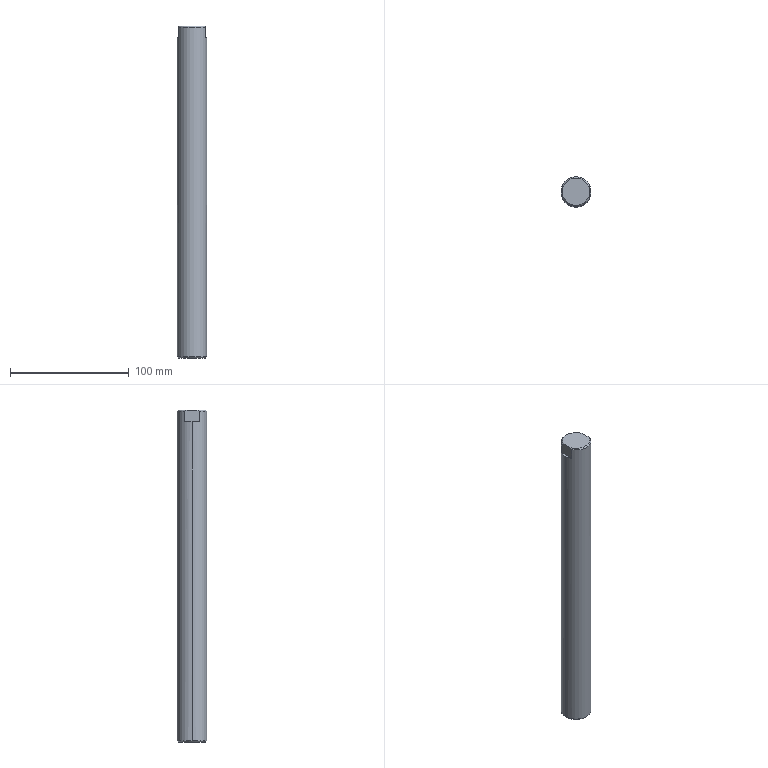Part | SolidWorks | features BaseBody 1 | 1 solid | 16 faces | box 25 x 25 x 280 mm | volume 136306 mm3 | cone 6 | plane 6 | cylinder 4 | commonest cylinder face diameters 6.8 x2 25 x2
STEP:
#1=CARTESIAN_POINT('',(3.4,0.,22.25));
#2=VERTEX_POINT('',#1);
#3=CARTESIAN_POINT('',(-3.4,0.,22.25));
#4=VERTEX_POINT('',#3);
#5=CARTESIAN_POINT('',(0.,0.,22.25));
#6=DIRECTION('',(0.,0.,-1.));
#7=DIRECTION('',(-1.,0.,0.));
#8=AXIS2_PLACEMENT_3D('',#5,#6,#7);
#9=CIRCLE('',#8,3.4);
#10=EDGE_CURVE('',#2,#4,#9,.T.);
#11=ORIENTED_EDGE('',*,*,#10,.F.);
#12=CARTESIAN_POINT('',(3.4,0.,0.));
#13=VERTEX_POINT('',#12);
#14=CARTESIAN_POINT('',(3.4,0.,0.));
#15=DIRECTION('',(0.,0.,-1.));
#16=VECTOR('',#15,1000.);
#17=LINE('',#14,#16);
#18=EDGE_CURVE('',#2,#13,#17,.T.);
#19=ORIENTED_EDGE('',*,*,#18,.T.);
#20=CARTESIAN_POINT('',(-3.4,0.,0.));
#21=VERTEX_POINT('',#20);
#22=CARTESIAN_POINT('',(0.,0.,0.));
#23=DIRECTION('',(0.,0.,-1.));
#24=DIRECTION('',(-1.,0.,0.));
#25=AXIS2_PLACEMENT_3D('',#22,#23,#24);
#26=CIRCLE('',#25,3.4);
#27=EDGE_CURVE('',#13,#21,#26,.T.);
#28=ORIENTED_EDGE('',*,*,#27,.T.);
#29=CARTESIAN_POINT('',(-3.4,0.,0.));
#30=DIRECTION('',(0.,0.,-1.));
#31=VECTOR('',#30,1000.);
#32=LINE('',#29,#31);
#33=EDGE_CURVE('',#4,#21,#32,.T.);
#34=ORIENTED_EDGE('',*,*,#33,.F.);
#35=EDGE_LOOP('',(#11,#19,#28,#34));
#36=FACE_OUTER_BOUND('',#35,.T.);
#37=CARTESIAN_POINT('',(0.,0.,0.));
#38=DIRECTION('',(0.,0.,-1.));
#39=DIRECTION('',(-1.,0.,0.));
#40=AXIS2_PLACEMENT_3D('',#37,#38,#39);
#41=CYLINDRICAL_SURFACE('',#40,3.4);
#42=ADVANCED_FACE('',(#36),#41,.F.);
#43=CARTESIAN_POINT('',(0.,0.,24.293));
#44=VERTEX_POINT('',#43);
#45=CARTESIAN_POINT('',(-3.4,0.,22.25));
#46=DIRECTION('',(-0.8572,0.,-0.515));
#47=VECTOR('',#46,1000.);
#48=LINE('',#45,#47);
#49=EDGE_CURVE('',#44,#4,#48,.T.);
#50=ORIENTED_EDGE('',*,*,#49,.F.);
#51=CARTESIAN_POINT('',(3.4,0.,22.25));
#52=DIRECTION('',(0.8572,0.,-0.515));
#53=VECTOR('',#52,1000.);
#54=LINE('',#51,#53);
#55=EDGE_CURVE('',#44,#2,#54,.T.);
#56=ORIENTED_EDGE('',*,*,#55,.T.);
#57=ORIENTED_EDGE('',*,*,#10,.T.);
#58=EDGE_LOOP('',(#50,#56,#57));
#59=FACE_OUTER_BOUND('',#58,.T.);
#60=CARTESIAN_POINT('',(0.,0.,22.25));
#61=DIRECTION('',(0.,0.,-1.));
#62=DIRECTION('',(-1.,0.,0.));
#63=AXIS2_PLACEMENT_3D('',#60,#61,#62);
#64=CONICAL_SURFACE('',#63,3.4,1.03);
#65=ADVANCED_FACE('',(#59),#64,.F.);
#66=CARTESIAN_POINT('',(-11.5,0.,0.));
#67=VERTEX_POINT('',#66);
#68=CARTESIAN_POINT('',(11.5,0.,0.));
#69=VERTEX_POINT('',#68);
#70=CARTESIAN_POINT('',(0.,0.,0.));
#71=DIRECTION('',(0.,0.,-1.));
#72=DIRECTION('',(1.,0.,0.));
#73=AXIS2_PLACEMENT_3D('',#70,#71,#72);
#74=CIRCLE('',#73,11.5);
#75=EDGE_CURVE('',#67,#69,#74,.T.);
#76=ORIENTED_EDGE('',*,*,#75,.F.);
#77=CARTESIAN_POINT('',(-12.5,0.,1.));
#78=VERTEX_POINT('',#77);
#79=CARTESIAN_POINT('',(-12.5,0.,1.));
#80=DIRECTION('',(-0.7071,0.,0.7071));
#81=VECTOR('',#80,1000.);
#82=LINE('',#79,#81);
#83=EDGE_CURVE('',#67,#78,#82,.T.);
#84=ORIENTED_EDGE('',*,*,#83,.T.);
#85=CARTESIAN_POINT('',(12.5,0.,1.));
#86=VERTEX_POINT('',#85);
#87=CARTESIAN_POINT('',(0.,0.,1.));
#88=DIRECTION('',(0.,0.,1.));
#89=DIRECTION('',(1.,0.,0.));
#90=AXIS2_PLACEMENT_3D('',#87,#88,#89);
#91=CIRCLE('',#90,12.5);
#92=EDGE_CURVE('',#86,#78,#91,.T.);
#93=ORIENTED_EDGE('',*,*,#92,.F.);
#94=CARTESIAN_POINT('',(12.5,0.,1.));
#95=DIRECTION('',(0.7071,0.,0.7071));
#96=VECTOR('',#95,1000.);
#97=LINE('',#94,#96);
#98=EDGE_CURVE('',#69,#86,#97,.T.);
#99=ORIENTED_EDGE('',*,*,#98,.F.);
#100=EDGE_LOOP('',(#76,#84,#93,#99));
#101=FACE_OUTER_BOUND('',#100,.T.);
#102=CARTESIAN_POINT('',(0.,0.,1.));
#103=DIRECTION('',(0.,0.,1.));
#104=DIRECTION('',(1.,0.,0.));
#105=AXIS2_PLACEMENT_3D('',#102,#103,#104);
#106=CONICAL_SURFACE('',#105,12.5,0.7854);
#107=ADVANCED_FACE('',(#101),#106,.T.);
#108=CARTESIAN_POINT('',(12.5,0.,270.));
#109=VERTEX_POINT('',#108);
#110=CARTESIAN_POINT('',(11.,5.937,270.));
#111=VERTEX_POINT('',#110);
#112=CARTESIAN_POINT('',(0.,0.,270.));
#113=DIRECTION('',(0.,0.,1.));
#114=DIRECTION('',(1.,0.,0.));
#115=AXIS2_PLACEMENT_3D('',#112,#113,#114);
#116=CIRCLE('',#115,12.5);
#117=EDGE_CURVE('',#109,#111,#116,.T.);
#118=ORIENTED_EDGE('',*,*,#117,.F.);
#119=CARTESIAN_POINT('',(12.5,0.,280.));
#120=DIRECTION('',(0.,0.,-1.));
#121=VECTOR('',#120,1000.);
#122=LINE('',#119,#121);
#123=EDGE_CURVE('',#109,#86,#122,.T.);
#124=ORIENTED_EDGE('',*,*,#123,.T.);
#125=ORIENTED_EDGE('',*,*,#92,.T.);
#126=CARTESIAN_POINT('',(-12.5,0.,270.));
#127=VERTEX_POINT('',#126);
#128=CARTESIAN_POINT('',(-12.5,0.,280.));
#129=DIRECTION('',(0.,0.,-1.));
#130=VECTOR('',#129,1000.);
#131=LINE('',#128,#130);
#132=EDGE_CURVE('',#127,#78,#131,.T.);
#133=ORIENTED_EDGE('',*,*,#132,.F.);
#134=CARTESIAN_POINT('',(-11.,5.937,270.));
#135=VERTEX_POINT('',#134);
#136=CARTESIAN_POINT('',(0.,0.,270.));
#137=DIRECTION('',(0.,0.,1.));
#138=DIRECTION('',(1.,0.,0.));
#139=AXIS2_PLACEMENT_3D('',#136,#137,#138);
#140=CIRCLE('',#139,12.5);
#141=EDGE_CURVE('',#135,#127,#140,.T.);
#142=ORIENTED_EDGE('',*,*,#141,.F.);
#143=CARTESIAN_POINT('',(-11.,5.937,279.));
#144=VERTEX_POINT('',#143);
#145=CARTESIAN_POINT('',(-11.,5.937,280.));
#146=DIRECTION('',(0.,0.,1.));
#147=VECTOR('',#146,1000.);
#148=LINE('',#145,#147);
#149=EDGE_CURVE('',#135,#144,#148,.T.);
#150=ORIENTED_EDGE('',*,*,#149,.T.);
#151=CARTESIAN_POINT('',(11.,5.937,279.));
#152=VERTEX_POINT('',#151);
#153=CARTESIAN_POINT('',(0.,0.,279.));
#154=DIRECTION('',(0.,0.,-1.));
#155=DIRECTION('',(1.,0.,0.));
#156=AXIS2_PLACEMENT_3D('',#153,#154,#155);
#157=CIRCLE('',#156,12.5);
#158=EDGE_CURVE('',#144,#152,#157,.T.);
#159=ORIENTED_EDGE('',*,*,#158,.T.);
#160=CARTESIAN_POINT('',(11.,5.937,280.));
#161=DIRECTION('',(0.,0.,-1.));
#162=VECTOR('',#161,1000.);
#163=LINE('',#160,#162);
#164=EDGE_CURVE('',#152,#111,#163,.T.);
#165=ORIENTED_EDGE('',*,*,#164,.T.);
#166=EDGE_LOOP('',(#118,#124,#125,#133,#142,#150,#159,#165));
#167=FACE_OUTER_BOUND('',#166,.T.);
#168=CARTESIAN_POINT('',(0.,0.,280.));
#169=DIRECTION('',(0.,0.,-1.));
#170=DIRECTION('',(-1.,0.,0.));
#171=AXIS2_PLACEMENT_3D('',#168,#169,#170);
#172=CYLINDRICAL_SURFACE('',#171,12.5);
#173=ADVANCED_FACE('',(#167),#172,.T.);
#174=CARTESIAN_POINT('',(11.,3.354,280.));
#175=VERTEX_POINT('',#174);
#176=CARTESIAN_POINT('',(11.,5.937,279.));
#177=CARTESIAN_POINT('',(11.,5.097,279.399));
#178=CARTESIAN_POINT('',(11.,4.239,279.742));
#179=CARTESIAN_POINT('',(11.,3.354,280.));
#180=B_SPLINE_CURVE_WITH_KNOTS('',3,(#176,#177,#178,#179),.UNSPECIFIED.,.F.,.F.,(4,4),(0.02005,0.02282),.UNSPECIFIED.);
#181=EDGE_CURVE('',#152,#175,#180,.T.);
#182=ORIENTED_EDGE('',*,*,#181,.F.);
#183=ORIENTED_EDGE('',*,*,#158,.F.);
#184=CARTESIAN_POINT('',(-11.,3.354,280.));
#185=VERTEX_POINT('',#184);
#186=CARTESIAN_POINT('',(-11.,3.354,280.));
#187=CARTESIAN_POINT('',(-11.,4.247,279.739));
#188=CARTESIAN_POINT('',(-11.,5.104,279.396));
#189=CARTESIAN_POINT('',(-11.,5.937,279.));
#190=B_SPLINE_CURVE_WITH_KNOTS('',3,(#186,#187,#188,#189),.UNSPECIFIED.,.F.,.F.,(4,4),(0.02963,0.03241),.UNSPECIFIED.);
#191=EDGE_CURVE('',#185,#144,#190,.T.);
#192=ORIENTED_EDGE('',*,*,#191,.F.);
#193=CARTESIAN_POINT('',(0.,0.,280.));
#194=DIRECTION('',(0.,0.,1.));
#195=DIRECTION('',(1.,0.,0.));
#196=AXIS2_PLACEMENT_3D('',#193,#194,#195);
#197=CIRCLE('',#196,11.5);
#198=EDGE_CURVE('',#175,#185,#197,.T.);
#199=ORIENTED_EDGE('',*,*,#198,.F.);
#200=EDGE_LOOP('',(#182,#183,#192,#199));
#201=FACE_OUTER_BOUND('',#200,.T.);
#202=CARTESIAN_POINT('',(0.,0.,280.));
#203=DIRECTION('',(0.,0.,-1.));
#204=DIRECTION('',(-1.,0.,0.));
#205=AXIS2_PLACEMENT_3D('',#202,#203,#204);
#206=CONICAL_SURFACE('',#205,11.5,0.7854);
#207=ADVANCED_FACE('',(#201),#206,.T.);
#208=ORIENTED_EDGE('',*,*,#123,.F.);
#209=CARTESIAN_POINT('',(11.,-5.937,270.));
#210=VERTEX_POINT('',#209);
#211=CARTESIAN_POINT('',(0.,0.,270.));
#212=DIRECTION('',(0.,0.,1.));
#213=DIRECTION('',(1.,0.,0.));
#214=AXIS2_PLACEMENT_3D('',#211,#212,#213);
#215=CIRCLE('',#214,12.5);
#216=EDGE_CURVE('',#210,#109,#215,.T.);
#217=ORIENTED_EDGE('',*,*,#216,.F.);
#218=CARTESIAN_POINT('',(11.,-5.937,279.));
#219=VERTEX_POINT('',#218);
#220=CARTESIAN_POINT('',(11.,-5.937,280.));
#221=DIRECTION('',(0.,0.,1.));
#222=VECTOR('',#221,1000.);
#223=LINE('',#220,#222);
#224=EDGE_CURVE('',#210,#219,#223,.T.);
#225=ORIENTED_EDGE('',*,*,#224,.T.);
#226=CARTESIAN_POINT('',(-11.,-5.937,279.));
#227=VERTEX_POINT('',#226);
#228=CARTESIAN_POINT('',(0.,0.,279.));
#229=DIRECTION('',(0.,0.,-1.));
#230=DIRECTION('',(1.,0.,0.));
#231=AXIS2_PLACEMENT_3D('',#228,#229,#230);
#232=CIRCLE('',#231,12.5);
#233=EDGE_CURVE('',#219,#227,#232,.T.);
#234=ORIENTED_EDGE('',*,*,#233,.T.);
#235=CARTESIAN_POINT('',(-11.,-5.937,270.));
#236=VERTEX_POINT('',#235);
#237=CARTESIAN_POINT('',(-11.,-5.937,280.));
#238=DIRECTION('',(0.,0.,-1.));
#239=VECTOR('',#238,1000.);
#240=LINE('',#237,#239);
#241=EDGE_CURVE('',#227,#236,#240,.T.);
#242=ORIENTED_EDGE('',*,*,#241,.T.);
#243=CARTESIAN_POINT('',(0.,0.,270.));
#244=DIRECTION('',(0.,0.,1.));
#245=DIRECTION('',(1.,0.,0.));
#246=AXIS2_PLACEMENT_3D('',#243,#244,#245);
#247=CIRCLE('',#246,12.5);
#248=EDGE_CURVE('',#127,#236,#247,.T.);
#249=ORIENTED_EDGE('',*,*,#248,.F.);
#250=ORIENTED_EDGE('',*,*,#132,.T.);
#251=CARTESIAN_POINT('',(0.,0.,1.));
#252=DIRECTION('',(0.,0.,1.));
#253=DIRECTION('',(1.,0.,0.));
#254=AXIS2_PLACEMENT_3D('',#251,#252,#253);
#255=CIRCLE('',#254,12.5);
#256=EDGE_CURVE('',#78,#86,#255,.T.);
#257=ORIENTED_EDGE('',*,*,#256,.T.);
#258=EDGE_LOOP('',(#208,#217,#225,#234,#242,#249,#250,#257));
#259=FACE_OUTER_BOUND('',#258,.T.);
#260=CARTESIAN_POINT('',(0.,0.,280.));
#261=DIRECTION('',(0.,0.,-1.));
#262=DIRECTION('',(-1.,0.,0.));
#263=AXIS2_PLACEMENT_3D('',#260,#261,#262);
#264=CYLINDRICAL_SURFACE('',#263,12.5);
#265=ADVANCED_FACE('',(#259),#264,.T.);
#266=CARTESIAN_POINT('',(11.,-3.354,280.));
#267=VERTEX_POINT('',#266);
#268=CARTESIAN_POINT('',(11.,10.,280.));
#269=DIRECTION('',(0.,-1.,0.));
#270=VECTOR('',#269,1000.);
#271=LINE('',#268,#270);
#272=EDGE_CURVE('',#175,#267,#271,.T.);
#273=ORIENTED_EDGE('',*,*,#272,.F.);
#274=ORIENTED_EDGE('',*,*,#198,.T.);
#275=CARTESIAN_POINT('',(-11.,-3.354,280.));
#276=VERTEX_POINT('',#275);
#277=CARTESIAN_POINT('',(-11.,10.,280.));
#278=DIRECTION('',(0.,1.,0.));
#279=VECTOR('',#278,1000.);
#280=LINE('',#277,#279);
#281=EDGE_CURVE('',#276,#185,#280,.T.);
#282=ORIENTED_EDGE('',*,*,#281,.F.);
#283=CARTESIAN_POINT('',(0.,0.,280.));
#284=DIRECTION('',(0.,0.,1.));
#285=DIRECTION('',(1.,0.,0.));
#286=AXIS2_PLACEMENT_3D('',#283,#284,#285);
#287=CIRCLE('',#286,11.5);
#288=EDGE_CURVE('',#276,#267,#287,.T.);
#289=ORIENTED_EDGE('',*,*,#288,.T.);
#290=EDGE_LOOP('',(#273,#274,#282,#289));
#291=FACE_OUTER_BOUND('',#290,.T.);
#292=CARTESIAN_POINT('',(0.,0.,280.));
#293=DIRECTION('',(0.,0.,1.));
#294=DIRECTION('',(1.,0.,0.));
#295=AXIS2_PLACEMENT_3D('',#292,#293,#294);
#296=PLANE('',#295);
#297=ADVANCED_FACE('',(#291),#296,.T.);
#298=CARTESIAN_POINT('',(0.,0.,0.));
#299=DIRECTION('',(0.,0.,-1.));
#300=DIRECTION('',(-1.,0.,0.));
#301=AXIS2_PLACEMENT_3D('',#298,#299,#300);
#302=CIRCLE('',#301,3.4);
#303=EDGE_CURVE('',#21,#13,#302,.T.);
#304=ORIENTED_EDGE('',*,*,#303,.F.);
#305=ORIENTED_EDGE('',*,*,#27,.F.);
#306=EDGE_LOOP('',(#304,#305));
#307=FACE_BOUND('',#306,.T.);
#308=CARTESIAN_POINT('',(0.,0.,0.));
#309=DIRECTION('',(0.,0.,-1.));
#310=DIRECTION('',(1.,0.,0.));
#311=AXIS2_PLACEMENT_3D('',#308,#309,#310);
#312=CIRCLE('',#311,11.5);
#313=EDGE_CURVE('',#69,#67,#312,.T.);
#314=ORIENTED_EDGE('',*,*,#313,.T.);
#315=ORIENTED_EDGE('',*,*,#75,.T.);
#316=EDGE_LOOP('',(#314,#315));
#317=FACE_OUTER_BOUND('',#316,.T.);
#318=CARTESIAN_POINT('',(0.,0.,0.));
#319=DIRECTION('',(0.,0.,1.));
#320=DIRECTION('',(1.,0.,0.));
#321=AXIS2_PLACEMENT_3D('',#318,#319,#320);
#322=PLANE('',#321);
#323=ADVANCED_FACE('',(#307,#317),#322,.F.);
#324=ORIENTED_EDGE('',*,*,#83,.F.);
#325=ORIENTED_EDGE('',*,*,#313,.F.);
#326=ORIENTED_EDGE('',*,*,#98,.T.);
#327=ORIENTED_EDGE('',*,*,#256,.F.);
#328=EDGE_LOOP('',(#324,#325,#326,#327));
#329=FACE_OUTER_BOUND('',#328,.T.);
#330=CARTESIAN_POINT('',(0.,0.,1.));
#331=DIRECTION('',(0.,0.,1.));
#332=DIRECTION('',(1.,0.,0.));
#333=AXIS2_PLACEMENT_3D('',#330,#331,#332);
#334=CONICAL_SURFACE('',#333,12.5,0.7854);
#335=ADVANCED_FACE('',(#329),#334,.T.);
#336=CARTESIAN_POINT('',(11.,-3.354,280.));
#337=CARTESIAN_POINT('',(11.,-4.247,279.739));
#338=CARTESIAN_POINT('',(11.,-5.104,279.396));
#339=CARTESIAN_POINT('',(11.,-5.937,279.));
#340=B_SPLINE_CURVE_WITH_KNOTS('',3,(#336,#337,#338,#339),.UNSPECIFIED.,.F.,.F.,(4,4),(0.02963,0.03241),.UNSPECIFIED.);
#341=EDGE_CURVE('',#267,#219,#340,.T.);
#342=ORIENTED_EDGE('',*,*,#341,.F.);
#343=ORIENTED_EDGE('',*,*,#288,.F.);
#344=CARTESIAN_POINT('',(-11.,-5.937,279.));
#345=CARTESIAN_POINT('',(-11.,-5.097,279.399));
#346=CARTESIAN_POINT('',(-11.,-4.239,279.742));
#347=CARTESIAN_POINT('',(-11.,-3.354,280.));
#348=B_SPLINE_CURVE_WITH_KNOTS('',3,(#344,#345,#346,#347),.UNSPECIFIED.,.F.,.F.,(4,4),(0.02005,0.02282),.UNSPECIFIED.);
#349=EDGE_CURVE('',#227,#276,#348,.T.);
#350=ORIENTED_EDGE('',*,*,#349,.F.);
#351=ORIENTED_EDGE('',*,*,#233,.F.);
#352=EDGE_LOOP('',(#342,#343,#350,#351));
#353=FACE_OUTER_BOUND('',#352,.T.);
#354=CARTESIAN_POINT('',(0.,0.,280.));
#355=DIRECTION('',(0.,0.,-1.));
#356=DIRECTION('',(-1.,0.,0.));
#357=AXIS2_PLACEMENT_3D('',#354,#355,#356);
#358=CONICAL_SURFACE('',#357,11.5,0.7854);
#359=ADVANCED_FACE('',(#353),#358,.T.);
#360=ORIENTED_EDGE('',*,*,#55,.F.);
#361=ORIENTED_EDGE('',*,*,#49,.T.);
#362=CARTESIAN_POINT('',(0.,0.,22.25));
#363=DIRECTION('',(0.,0.,-1.));
#364=DIRECTION('',(-1.,0.,0.));
#365=AXIS2_PLACEMENT_3D('',#362,#363,#364);
#366=CIRCLE('',#365,3.4);
#367=EDGE_CURVE('',#4,#2,#366,.T.);
#368=ORIENTED_EDGE('',*,*,#367,.T.);
#369=EDGE_LOOP('',(#360,#361,#368));
#370=FACE_OUTER_BOUND('',#369,.T.);
#371=CARTESIAN_POINT('',(0.,0.,22.25));
#372=DIRECTION('',(0.,0.,-1.));
#373=DIRECTION('',(-1.,0.,0.));
#374=AXIS2_PLACEMENT_3D('',#371,#372,#373);
#375=CONICAL_SURFACE('',#374,3.4,1.03);
#376=ADVANCED_FACE('',(#370),#375,.F.);
#377=ORIENTED_EDGE('',*,*,#18,.F.);
#378=ORIENTED_EDGE('',*,*,#367,.F.);
#379=ORIENTED_EDGE('',*,*,#33,.T.);
#380=ORIENTED_EDGE('',*,*,#303,.T.);
#381=EDGE_LOOP('',(#377,#378,#379,#380));
#382=FACE_OUTER_BOUND('',#381,.T.);
#383=CARTESIAN_POINT('',(0.,0.,0.));
#384=DIRECTION('',(0.,0.,-1.));
#385=DIRECTION('',(-1.,0.,0.));
#386=AXIS2_PLACEMENT_3D('',#383,#384,#385);
#387=CYLINDRICAL_SURFACE('',#386,3.4);
#388=ADVANCED_FACE('',(#382),#387,.F.);
#389=ORIENTED_EDGE('',*,*,#141,.T.);
#390=ORIENTED_EDGE('',*,*,#248,.T.);
#391=CARTESIAN_POINT('',(-11.,10.,270.));
#392=DIRECTION('',(0.,1.,0.));
#393=VECTOR('',#392,1000.);
#394=LINE('',#391,#393);
#395=EDGE_CURVE('',#236,#135,#394,.T.);
#396=ORIENTED_EDGE('',*,*,#395,.T.);
#397=EDGE_LOOP('',(#389,#390,#396));
#398=FACE_OUTER_BOUND('',#397,.T.);
#399=CARTESIAN_POINT('',(0.,0.,270.));
#400=DIRECTION('',(0.,0.,1.));
#401=DIRECTION('',(1.,0.,0.));
#402=AXIS2_PLACEMENT_3D('',#399,#400,#401);
#403=PLANE('',#402);
#404=ADVANCED_FACE('',(#398),#403,.T.);
#405=ORIENTED_EDGE('',*,*,#349,.T.);
#406=ORIENTED_EDGE('',*,*,#281,.T.);
#407=ORIENTED_EDGE('',*,*,#191,.T.);
#408=ORIENTED_EDGE('',*,*,#149,.F.);
#409=ORIENTED_EDGE('',*,*,#395,.F.);
#410=ORIENTED_EDGE('',*,*,#241,.F.);
#411=EDGE_LOOP('',(#405,#406,#407,#408,#409,#410));
#412=FACE_OUTER_BOUND('',#411,.T.);
#413=CARTESIAN_POINT('',(-11.,10.,270.));
#414=DIRECTION('',(1.,0.,0.));
#415=DIRECTION('',(0.,1.,0.));
#416=AXIS2_PLACEMENT_3D('',#413,#414,#415);
#417=PLANE('',#416);
#418=ADVANCED_FACE('',(#412),#417,.F.);
#419=ORIENTED_EDGE('',*,*,#216,.T.);
#420=ORIENTED_EDGE('',*,*,#117,.T.);
#421=CARTESIAN_POINT('',(11.,10.,270.));
#422=DIRECTION('',(0.,-1.,0.));
#423=VECTOR('',#422,1000.);
#424=LINE('',#421,#423);
#425=EDGE_CURVE('',#111,#210,#424,.T.);
#426=ORIENTED_EDGE('',*,*,#425,.T.);
#427=EDGE_LOOP('',(#419,#420,#426));
#428=FACE_OUTER_BOUND('',#427,.T.);
#429=CARTESIAN_POINT('',(0.,0.,270.));
#430=DIRECTION('',(0.,0.,1.));
#431=DIRECTION('',(1.,0.,0.));
#432=AXIS2_PLACEMENT_3D('',#429,#430,#431);
#433=PLANE('',#432);
#434=ADVANCED_FACE('',(#428),#433,.T.);
#435=ORIENTED_EDGE('',*,*,#181,.T.);
#436=ORIENTED_EDGE('',*,*,#272,.T.);
#437=ORIENTED_EDGE('',*,*,#341,.T.);
#438=ORIENTED_EDGE('',*,*,#224,.F.);
#439=ORIENTED_EDGE('',*,*,#425,.F.);
#440=ORIENTED_EDGE('',*,*,#164,.F.);
#441=EDGE_LOOP('',(#435,#436,#437,#438,#439,#440));
#442=FACE_OUTER_BOUND('',#441,.T.);
#443=CARTESIAN_POINT('',(11.,10.,270.));
#444=DIRECTION('',(-1.,0.,0.));
#445=DIRECTION('',(0.,-1.,0.));
#446=AXIS2_PLACEMENT_3D('',#443,#444,#445);
#447=PLANE('',#446);
#448=ADVANCED_FACE('',(#442),#447,.F.);
#449=CLOSED_SHELL('',(#42,#65,#107,#173,#207,#265,#297,#323,#335,#359,#376,#388,#404,#418,#434,#448));
#450=MANIFOLD_SOLID_BREP('',#449);
#451=CARTESIAN_POINT('',(0.,0.,0.));
#452=DIRECTION('',(0.,0.,1.));
#453=DIRECTION('',(1.,0.,0.));
#454=AXIS2_PLACEMENT_3D('',#451,#452,#453);
#455=(LENGTH_UNIT()NAMED_UNIT(*)SI_UNIT(.MILLI.,.METRE.));
#456=UNCERTAINTY_MEASURE_WITH_UNIT(LENGTH_MEASURE(0.00001),#455,'','');
#457=(NAMED_UNIT(*)PLANE_ANGLE_UNIT()SI_UNIT($,.RADIAN.));
#458=(NAMED_UNIT(*)SI_UNIT($,.STERADIAN.)SOLID_ANGLE_UNIT());
#459=(GEOMETRIC_REPRESENTATION_CONTEXT(3)GLOBAL_UNCERTAINTY_ASSIGNED_CONTEXT((#456))GLOBAL_UNIT_ASSIGNED_CONTEXT((#455,#457,#458))REPRESENTATION_CONTEXT('',''));
#460=ADVANCED_BREP_SHAPE_REPRESENTATION('',(#450,#454),#459);